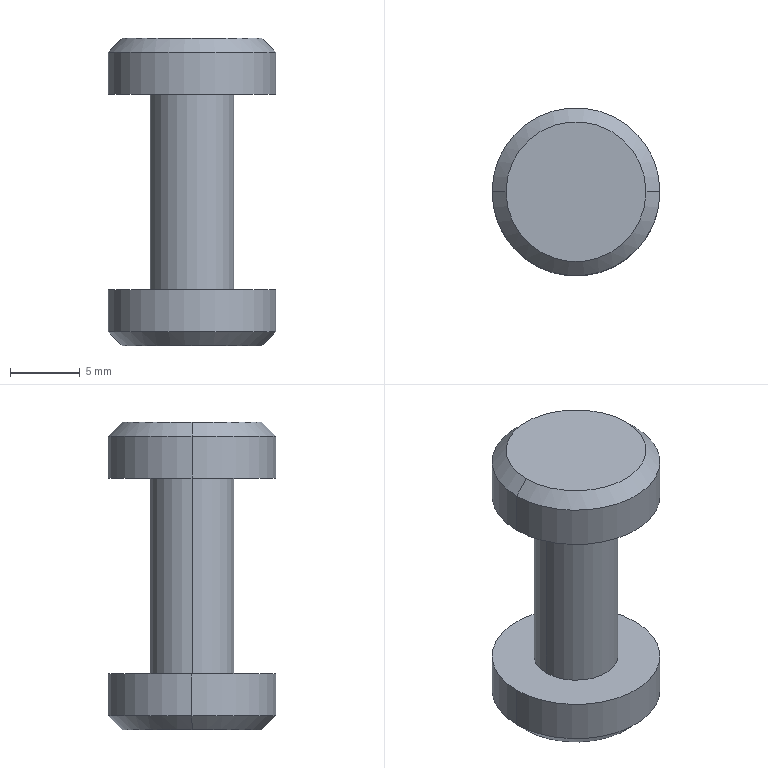Part | SolidWorks | features Chamfer 2, ICE 2, Extrusion 1 | 1 solid | 14 faces | box 12 x 12 x 22 mm | volume 1265 mm3 | cylinder 6 | cone 4 | plane 4 | commonest cylinder face diameters 12 x4 6 x2
STEP:
#1=CARTESIAN_POINT('',(-5.,0.,-4.));
#2=VERTEX_POINT('',#1);
#3=CARTESIAN_POINT('',(5.,0.,-4.));
#4=VERTEX_POINT('',#3);
#5=CARTESIAN_POINT('',(0.,0.,-4.));
#6=DIRECTION('',(0.,0.,-1.));
#7=DIRECTION('',(-1.,0.,0.));
#8=AXIS2_PLACEMENT_3D('',#5,#6,#7);
#9=CIRCLE('',#8,5.);
#10=EDGE_CURVE('',#2,#4,#9,.T.);
#11=ORIENTED_EDGE('',*,*,#10,.F.);
#12=CARTESIAN_POINT('',(-6.,0.,-3.));
#13=VERTEX_POINT('',#12);
#14=CARTESIAN_POINT('',(-5.,0.,-4.));
#15=DIRECTION('',(-0.7071,0.,0.7071));
#16=VECTOR('',#15,1000.);
#17=LINE('',#14,#16);
#18=EDGE_CURVE('',#2,#13,#17,.T.);
#19=ORIENTED_EDGE('',*,*,#18,.T.);
#20=CARTESIAN_POINT('',(6.,0.,-3.));
#21=VERTEX_POINT('',#20);
#22=CARTESIAN_POINT('',(0.,0.,-3.));
#23=DIRECTION('',(0.,0.,1.));
#24=DIRECTION('',(-1.,0.,0.));
#25=AXIS2_PLACEMENT_3D('',#22,#23,#24);
#26=CIRCLE('',#25,6.);
#27=EDGE_CURVE('',#21,#13,#26,.T.);
#28=ORIENTED_EDGE('',*,*,#27,.F.);
#29=CARTESIAN_POINT('',(5.,0.,-4.));
#30=DIRECTION('',(0.7071,0.,0.7071));
#31=VECTOR('',#30,1000.);
#32=LINE('',#29,#31);
#33=EDGE_CURVE('',#4,#21,#32,.T.);
#34=ORIENTED_EDGE('',*,*,#33,.F.);
#35=EDGE_LOOP('',(#11,#19,#28,#34));
#36=FACE_OUTER_BOUND('',#35,.T.);
#37=CARTESIAN_POINT('',(0.,0.,-4.));
#38=DIRECTION('',(0.,0.,1.));
#39=DIRECTION('',(1.,0.,0.));
#40=AXIS2_PLACEMENT_3D('',#37,#38,#39);
#41=CONICAL_SURFACE('',#40,5.,0.7854);
#42=ADVANCED_FACE('',(#36),#41,.T.);
#43=ORIENTED_EDGE('',*,*,#27,.T.);
#44=CARTESIAN_POINT('',(-6.,0.,0.));
#45=VERTEX_POINT('',#44);
#46=CARTESIAN_POINT('',(-6.,0.,-4.));
#47=DIRECTION('',(0.,0.,1.));
#48=VECTOR('',#47,1000.);
#49=LINE('',#46,#48);
#50=EDGE_CURVE('',#13,#45,#49,.T.);
#51=ORIENTED_EDGE('',*,*,#50,.T.);
#52=CARTESIAN_POINT('',(6.,0.,0.));
#53=VERTEX_POINT('',#52);
#54=CARTESIAN_POINT('',(0.,0.,0.));
#55=DIRECTION('',(0.,0.,-1.));
#56=DIRECTION('',(-1.,0.,0.));
#57=AXIS2_PLACEMENT_3D('',#54,#55,#56);
#58=CIRCLE('',#57,6.);
#59=EDGE_CURVE('',#45,#53,#58,.T.);
#60=ORIENTED_EDGE('',*,*,#59,.T.);
#61=CARTESIAN_POINT('',(6.,0.,-4.));
#62=DIRECTION('',(0.,0.,1.));
#63=VECTOR('',#62,1000.);
#64=LINE('',#61,#63);
#65=EDGE_CURVE('',#21,#53,#64,.T.);
#66=ORIENTED_EDGE('',*,*,#65,.F.);
#67=EDGE_LOOP('',(#43,#51,#60,#66));
#68=FACE_OUTER_BOUND('',#67,.T.);
#69=CARTESIAN_POINT('',(0.,0.,-4.));
#70=DIRECTION('',(0.,0.,1.));
#71=DIRECTION('',(1.,0.,0.));
#72=AXIS2_PLACEMENT_3D('',#69,#70,#71);
#73=CYLINDRICAL_SURFACE('',#72,6.);
#74=ADVANCED_FACE('',(#68),#73,.T.);
#75=CARTESIAN_POINT('',(5.,0.,18.));
#76=VERTEX_POINT('',#75);
#77=CARTESIAN_POINT('',(-5.,0.,18.));
#78=VERTEX_POINT('',#77);
#79=CARTESIAN_POINT('',(0.,0.,18.));
#80=DIRECTION('',(0.,0.,1.));
#81=DIRECTION('',(1.,0.,0.));
#82=AXIS2_PLACEMENT_3D('',#79,#80,#81);
#83=CIRCLE('',#82,5.);
#84=EDGE_CURVE('',#76,#78,#83,.T.);
#85=ORIENTED_EDGE('',*,*,#84,.F.);
#86=CARTESIAN_POINT('',(6.,0.,17.));
#87=VERTEX_POINT('',#86);
#88=CARTESIAN_POINT('',(5.,0.,18.));
#89=DIRECTION('',(0.7071,0.,-0.7071));
#90=VECTOR('',#89,1000.);
#91=LINE('',#88,#90);
#92=EDGE_CURVE('',#76,#87,#91,.T.);
#93=ORIENTED_EDGE('',*,*,#92,.T.);
#94=CARTESIAN_POINT('',(-6.,0.,17.));
#95=VERTEX_POINT('',#94);
#96=CARTESIAN_POINT('',(0.,0.,17.));
#97=DIRECTION('',(0.,0.,-1.));
#98=DIRECTION('',(1.,0.,0.));
#99=AXIS2_PLACEMENT_3D('',#96,#97,#98);
#100=CIRCLE('',#99,6.);
#101=EDGE_CURVE('',#95,#87,#100,.T.);
#102=ORIENTED_EDGE('',*,*,#101,.F.);
#103=CARTESIAN_POINT('',(-5.,0.,18.));
#104=DIRECTION('',(-0.7071,0.,-0.7071));
#105=VECTOR('',#104,1000.);
#106=LINE('',#103,#105);
#107=EDGE_CURVE('',#78,#95,#106,.T.);
#108=ORIENTED_EDGE('',*,*,#107,.F.);
#109=EDGE_LOOP('',(#85,#93,#102,#108));
#110=FACE_OUTER_BOUND('',#109,.T.);
#111=CARTESIAN_POINT('',(0.,0.,18.));
#112=DIRECTION('',(0.,0.,-1.));
#113=DIRECTION('',(-1.,0.,0.));
#114=AXIS2_PLACEMENT_3D('',#111,#112,#113);
#115=CONICAL_SURFACE('',#114,5.,0.7854);
#116=ADVANCED_FACE('',(#110),#115,.T.);
#117=ORIENTED_EDGE('',*,*,#101,.T.);
#118=CARTESIAN_POINT('',(6.,0.,14.));
#119=VERTEX_POINT('',#118);
#120=CARTESIAN_POINT('',(6.,0.,18.));
#121=DIRECTION('',(0.,0.,-1.));
#122=VECTOR('',#121,1000.);
#123=LINE('',#120,#122);
#124=EDGE_CURVE('',#87,#119,#123,.T.);
#125=ORIENTED_EDGE('',*,*,#124,.T.);
#126=CARTESIAN_POINT('',(-6.,0.,14.));
#127=VERTEX_POINT('',#126);
#128=CARTESIAN_POINT('',(0.,0.,14.));
#129=DIRECTION('',(0.,0.,1.));
#130=DIRECTION('',(1.,0.,0.));
#131=AXIS2_PLACEMENT_3D('',#128,#129,#130);
#132=CIRCLE('',#131,6.);
#133=EDGE_CURVE('',#119,#127,#132,.T.);
#134=ORIENTED_EDGE('',*,*,#133,.T.);
#135=CARTESIAN_POINT('',(-6.,0.,18.));
#136=DIRECTION('',(0.,0.,-1.));
#137=VECTOR('',#136,1000.);
#138=LINE('',#135,#137);
#139=EDGE_CURVE('',#95,#127,#138,.T.);
#140=ORIENTED_EDGE('',*,*,#139,.F.);
#141=EDGE_LOOP('',(#117,#125,#134,#140));
#142=FACE_OUTER_BOUND('',#141,.T.);
#143=CARTESIAN_POINT('',(0.,0.,18.));
#144=DIRECTION('',(0.,0.,-1.));
#145=DIRECTION('',(-1.,0.,0.));
#146=AXIS2_PLACEMENT_3D('',#143,#144,#145);
#147=CYLINDRICAL_SURFACE('',#146,6.);
#148=ADVANCED_FACE('',(#142),#147,.T.);
#149=CARTESIAN_POINT('',(3.,0.,14.));
#150=VERTEX_POINT('',#149);
#151=CARTESIAN_POINT('',(-3.,0.,14.));
#152=VERTEX_POINT('',#151);
#153=CARTESIAN_POINT('',(0.,0.,14.));
#154=DIRECTION('',(0.,0.,1.));
#155=DIRECTION('',(1.,0.,0.));
#156=AXIS2_PLACEMENT_3D('',#153,#154,#155);
#157=CIRCLE('',#156,3.);
#158=EDGE_CURVE('',#150,#152,#157,.T.);
#159=ORIENTED_EDGE('',*,*,#158,.F.);
#160=CARTESIAN_POINT('',(3.,0.,0.));
#161=VERTEX_POINT('',#160);
#162=CARTESIAN_POINT('',(3.,0.,14.));
#163=DIRECTION('',(0.,0.,-1.));
#164=VECTOR('',#163,1000.);
#165=LINE('',#162,#164);
#166=EDGE_CURVE('',#150,#161,#165,.T.);
#167=ORIENTED_EDGE('',*,*,#166,.T.);
#168=CARTESIAN_POINT('',(-3.,0.,0.));
#169=VERTEX_POINT('',#168);
#170=CARTESIAN_POINT('',(0.,0.,0.));
#171=DIRECTION('',(0.,0.,1.));
#172=DIRECTION('',(1.,0.,0.));
#173=AXIS2_PLACEMENT_3D('',#170,#171,#172);
#174=CIRCLE('',#173,3.);
#175=EDGE_CURVE('',#161,#169,#174,.T.);
#176=ORIENTED_EDGE('',*,*,#175,.T.);
#177=CARTESIAN_POINT('',(-3.,0.,14.));
#178=DIRECTION('',(0.,0.,-1.));
#179=VECTOR('',#178,1000.);
#180=LINE('',#177,#179);
#181=EDGE_CURVE('',#152,#169,#180,.T.);
#182=ORIENTED_EDGE('',*,*,#181,.F.);
#183=EDGE_LOOP('',(#159,#167,#176,#182));
#184=FACE_OUTER_BOUND('',#183,.T.);
#185=CARTESIAN_POINT('',(0.,0.,14.));
#186=DIRECTION('',(0.,0.,-1.));
#187=DIRECTION('',(-1.,0.,0.));
#188=AXIS2_PLACEMENT_3D('',#185,#186,#187);
#189=CYLINDRICAL_SURFACE('',#188,3.);
#190=ADVANCED_FACE('',(#184),#189,.T.);
#191=ORIENTED_EDGE('',*,*,#166,.F.);
#192=CARTESIAN_POINT('',(0.,0.,14.));
#193=DIRECTION('',(0.,0.,1.));
#194=DIRECTION('',(1.,0.,0.));
#195=AXIS2_PLACEMENT_3D('',#192,#193,#194);
#196=CIRCLE('',#195,3.);
#197=EDGE_CURVE('',#152,#150,#196,.T.);
#198=ORIENTED_EDGE('',*,*,#197,.F.);
#199=ORIENTED_EDGE('',*,*,#181,.T.);
#200=CARTESIAN_POINT('',(0.,0.,0.));
#201=DIRECTION('',(0.,0.,1.));
#202=DIRECTION('',(1.,0.,0.));
#203=AXIS2_PLACEMENT_3D('',#200,#201,#202);
#204=CIRCLE('',#203,3.);
#205=EDGE_CURVE('',#169,#161,#204,.T.);
#206=ORIENTED_EDGE('',*,*,#205,.T.);
#207=EDGE_LOOP('',(#191,#198,#199,#206));
#208=FACE_OUTER_BOUND('',#207,.T.);
#209=CARTESIAN_POINT('',(0.,0.,14.));
#210=DIRECTION('',(0.,0.,-1.));
#211=DIRECTION('',(-1.,0.,0.));
#212=AXIS2_PLACEMENT_3D('',#209,#210,#211);
#213=CYLINDRICAL_SURFACE('',#212,3.);
#214=ADVANCED_FACE('',(#208),#213,.T.);
#215=ORIENTED_EDGE('',*,*,#124,.F.);
#216=CARTESIAN_POINT('',(0.,0.,17.));
#217=DIRECTION('',(0.,0.,-1.));
#218=DIRECTION('',(1.,0.,0.));
#219=AXIS2_PLACEMENT_3D('',#216,#217,#218);
#220=CIRCLE('',#219,6.);
#221=EDGE_CURVE('',#87,#95,#220,.T.);
#222=ORIENTED_EDGE('',*,*,#221,.T.);
#223=ORIENTED_EDGE('',*,*,#139,.T.);
#224=CARTESIAN_POINT('',(0.,0.,14.));
#225=DIRECTION('',(0.,0.,1.));
#226=DIRECTION('',(1.,0.,0.));
#227=AXIS2_PLACEMENT_3D('',#224,#225,#226);
#228=CIRCLE('',#227,6.);
#229=EDGE_CURVE('',#127,#119,#228,.T.);
#230=ORIENTED_EDGE('',*,*,#229,.T.);
#231=EDGE_LOOP('',(#215,#222,#223,#230));
#232=FACE_OUTER_BOUND('',#231,.T.);
#233=CARTESIAN_POINT('',(0.,0.,18.));
#234=DIRECTION('',(0.,0.,-1.));
#235=DIRECTION('',(-1.,0.,0.));
#236=AXIS2_PLACEMENT_3D('',#233,#234,#235);
#237=CYLINDRICAL_SURFACE('',#236,6.);
#238=ADVANCED_FACE('',(#232),#237,.T.);
#239=CARTESIAN_POINT('',(0.,0.,18.));
#240=DIRECTION('',(0.,0.,1.));
#241=DIRECTION('',(1.,0.,0.));
#242=AXIS2_PLACEMENT_3D('',#239,#240,#241);
#243=CIRCLE('',#242,5.);
#244=EDGE_CURVE('',#78,#76,#243,.T.);
#245=ORIENTED_EDGE('',*,*,#244,.T.);
#246=ORIENTED_EDGE('',*,*,#84,.T.);
#247=EDGE_LOOP('',(#245,#246));
#248=FACE_OUTER_BOUND('',#247,.T.);
#249=CARTESIAN_POINT('',(0.,0.,18.));
#250=DIRECTION('',(0.,0.,1.));
#251=DIRECTION('',(1.,0.,0.));
#252=AXIS2_PLACEMENT_3D('',#249,#250,#251);
#253=PLANE('',#252);
#254=ADVANCED_FACE('',(#248),#253,.T.);
#255=ORIENTED_EDGE('',*,*,#197,.T.);
#256=ORIENTED_EDGE('',*,*,#158,.T.);
#257=EDGE_LOOP('',(#255,#256));
#258=FACE_BOUND('',#257,.T.);
#259=ORIENTED_EDGE('',*,*,#229,.F.);
#260=ORIENTED_EDGE('',*,*,#133,.F.);
#261=EDGE_LOOP('',(#259,#260));
#262=FACE_OUTER_BOUND('',#261,.T.);
#263=CARTESIAN_POINT('',(0.,0.,14.));
#264=DIRECTION('',(0.,0.,1.));
#265=DIRECTION('',(1.,0.,0.));
#266=AXIS2_PLACEMENT_3D('',#263,#264,#265);
#267=PLANE('',#266);
#268=ADVANCED_FACE('',(#258,#262),#267,.F.);
#269=ORIENTED_EDGE('',*,*,#92,.F.);
#270=ORIENTED_EDGE('',*,*,#244,.F.);
#271=ORIENTED_EDGE('',*,*,#107,.T.);
#272=ORIENTED_EDGE('',*,*,#221,.F.);
#273=EDGE_LOOP('',(#269,#270,#271,#272));
#274=FACE_OUTER_BOUND('',#273,.T.);
#275=CARTESIAN_POINT('',(0.,0.,18.));
#276=DIRECTION('',(0.,0.,-1.));
#277=DIRECTION('',(-1.,0.,0.));
#278=AXIS2_PLACEMENT_3D('',#275,#276,#277);
#279=CONICAL_SURFACE('',#278,5.,0.7854);
#280=ADVANCED_FACE('',(#274),#279,.T.);
#281=ORIENTED_EDGE('',*,*,#50,.F.);
#282=CARTESIAN_POINT('',(0.,0.,-3.));
#283=DIRECTION('',(0.,0.,1.));
#284=DIRECTION('',(-1.,0.,0.));
#285=AXIS2_PLACEMENT_3D('',#282,#283,#284);
#286=CIRCLE('',#285,6.);
#287=EDGE_CURVE('',#13,#21,#286,.T.);
#288=ORIENTED_EDGE('',*,*,#287,.T.);
#289=ORIENTED_EDGE('',*,*,#65,.T.);
#290=CARTESIAN_POINT('',(0.,0.,0.));
#291=DIRECTION('',(0.,0.,-1.));
#292=DIRECTION('',(-1.,0.,0.));
#293=AXIS2_PLACEMENT_3D('',#290,#291,#292);
#294=CIRCLE('',#293,6.);
#295=EDGE_CURVE('',#53,#45,#294,.T.);
#296=ORIENTED_EDGE('',*,*,#295,.T.);
#297=EDGE_LOOP('',(#281,#288,#289,#296));
#298=FACE_OUTER_BOUND('',#297,.T.);
#299=CARTESIAN_POINT('',(0.,0.,-4.));
#300=DIRECTION('',(0.,0.,1.));
#301=DIRECTION('',(1.,0.,0.));
#302=AXIS2_PLACEMENT_3D('',#299,#300,#301);
#303=CYLINDRICAL_SURFACE('',#302,6.);
#304=ADVANCED_FACE('',(#298),#303,.T.);
#305=CARTESIAN_POINT('',(0.,0.,-4.));
#306=DIRECTION('',(0.,0.,-1.));
#307=DIRECTION('',(-1.,0.,0.));
#308=AXIS2_PLACEMENT_3D('',#305,#306,#307);
#309=CIRCLE('',#308,5.);
#310=EDGE_CURVE('',#4,#2,#309,.T.);
#311=ORIENTED_EDGE('',*,*,#310,.T.);
#312=ORIENTED_EDGE('',*,*,#10,.T.);
#313=EDGE_LOOP('',(#311,#312));
#314=FACE_OUTER_BOUND('',#313,.T.);
#315=CARTESIAN_POINT('',(0.,0.,-4.));
#316=DIRECTION('',(0.,0.,-1.));
#317=DIRECTION('',(-1.,0.,0.));
#318=AXIS2_PLACEMENT_3D('',#315,#316,#317);
#319=PLANE('',#318);
#320=ADVANCED_FACE('',(#314),#319,.T.);
#321=ORIENTED_EDGE('',*,*,#205,.F.);
#322=ORIENTED_EDGE('',*,*,#175,.F.);
#323=EDGE_LOOP('',(#321,#322));
#324=FACE_BOUND('',#323,.T.);
#325=ORIENTED_EDGE('',*,*,#295,.F.);
#326=ORIENTED_EDGE('',*,*,#59,.F.);
#327=EDGE_LOOP('',(#325,#326));
#328=FACE_OUTER_BOUND('',#327,.T.);
#329=CARTESIAN_POINT('',(0.,0.,0.));
#330=DIRECTION('',(0.,0.,-1.));
#331=DIRECTION('',(-1.,0.,0.));
#332=AXIS2_PLACEMENT_3D('',#329,#330,#331);
#333=PLANE('',#332);
#334=ADVANCED_FACE('',(#324,#328),#333,.F.);
#335=ORIENTED_EDGE('',*,*,#18,.F.);
#336=ORIENTED_EDGE('',*,*,#310,.F.);
#337=ORIENTED_EDGE('',*,*,#33,.T.);
#338=ORIENTED_EDGE('',*,*,#287,.F.);
#339=EDGE_LOOP('',(#335,#336,#337,#338));
#340=FACE_OUTER_BOUND('',#339,.T.);
#341=CARTESIAN_POINT('',(0.,0.,-4.));
#342=DIRECTION('',(0.,0.,1.));
#343=DIRECTION('',(1.,0.,0.));
#344=AXIS2_PLACEMENT_3D('',#341,#342,#343);
#345=CONICAL_SURFACE('',#344,5.,0.7854);
#346=ADVANCED_FACE('',(#340),#345,.T.);
#347=CLOSED_SHELL('',(#42,#74,#116,#148,#190,#214,#238,#254,#268,#280,#304,#320,#334,#346));
#348=MANIFOLD_SOLID_BREP('',#347);
#349=CARTESIAN_POINT('',(0.,0.,0.));
#350=DIRECTION('',(0.,0.,1.));
#351=DIRECTION('',(1.,0.,0.));
#352=AXIS2_PLACEMENT_3D('',#349,#350,#351);
#353=(LENGTH_UNIT()NAMED_UNIT(*)SI_UNIT(.MILLI.,.METRE.));
#354=UNCERTAINTY_MEASURE_WITH_UNIT(LENGTH_MEASURE(0.00001),#353,'','');
#355=(NAMED_UNIT(*)PLANE_ANGLE_UNIT()SI_UNIT($,.RADIAN.));
#356=(NAMED_UNIT(*)SI_UNIT($,.STERADIAN.)SOLID_ANGLE_UNIT());
#357=(GEOMETRIC_REPRESENTATION_CONTEXT(3)GLOBAL_UNCERTAINTY_ASSIGNED_CONTEXT((#354))GLOBAL_UNIT_ASSIGNED_CONTEXT((#353,#355,#356))REPRESENTATION_CONTEXT('',''));
#358=ADVANCED_BREP_SHAPE_REPRESENTATION('',(#348,#352),#357);